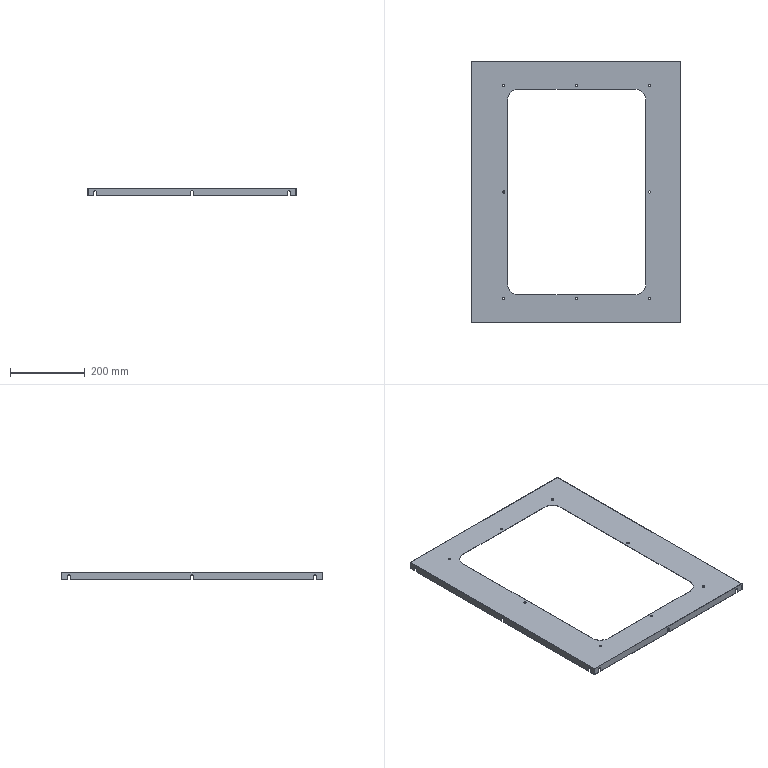Part | STEP file | PN_0017 | 1 solid | 88 faces | box 558 x 698 x 20 mm | volume 233111 mm3 | plane 50 | cylinder 38 | commonest cylinder face diameters 7 x18 6 x16 60 x4